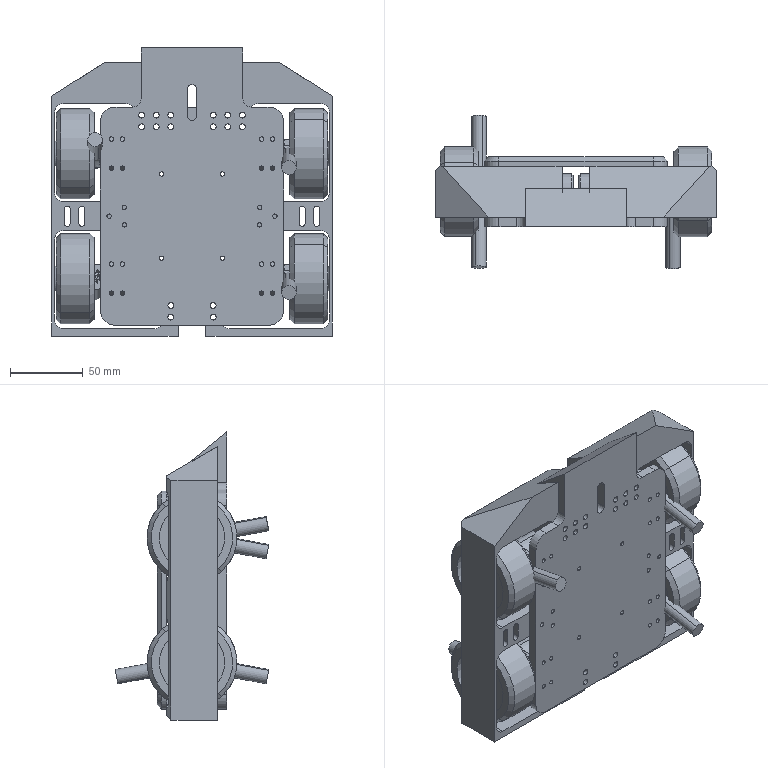Part | SolidWorks | 28 solids | 1163 faces | box 193.215 x 105.647 x 198.21 mm | volume 922670 mm3 | cylinder 561 | plane 534 | cone 68 | commonest cylinder face diameters 3 x232 4 x112 3.593 x40 0.6 x32 10 x16 17.78 x16